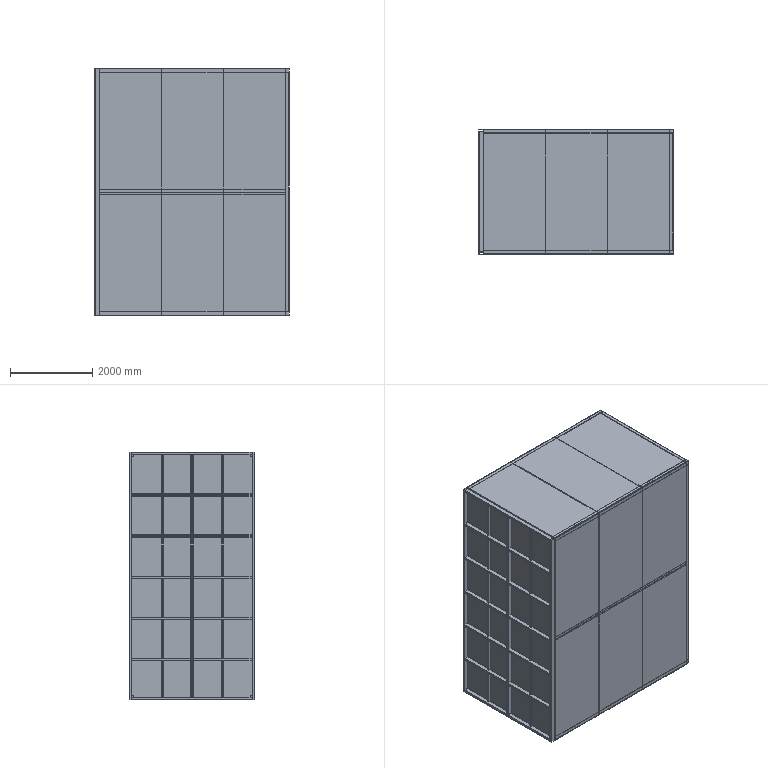Part | SolidWorks | features ReferencePattern 20, LocalLPattern 7, LayoutProfileFeature 1 | 37 solids | 490 faces | box 4720 x 3046 x 6011 mm | volume 585161679 mm3 | plane 314 | cylinder 176 | commonest cylinder face diameters 10 x88 20 x76 5 x8 4 x4